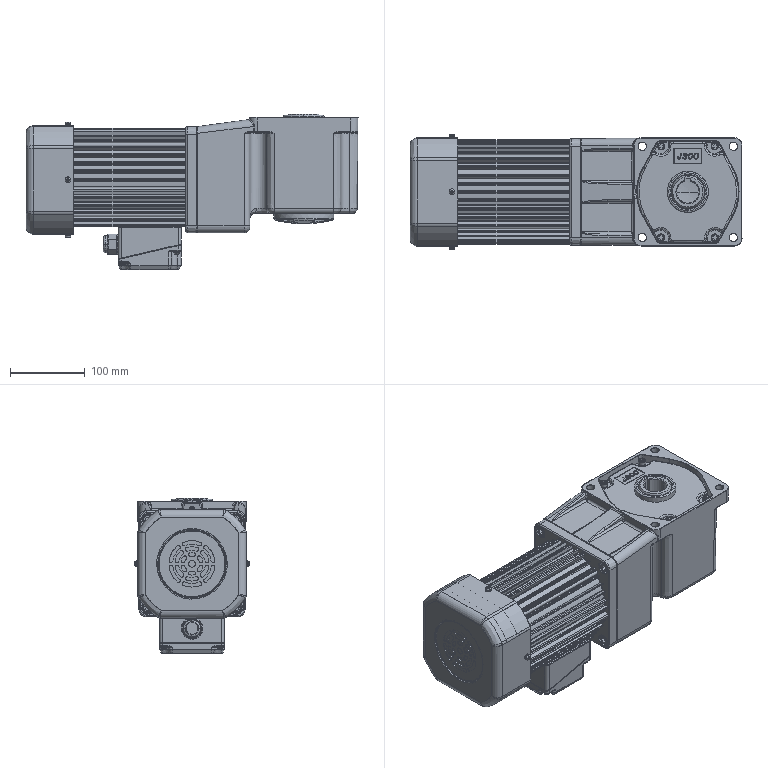Part | STEP file | s750rc-U | 4 solids | 3526 faces | volume 5609613 mm3 | spline 1255 | cylinder 1248 | plane 933 | cone 73 | torus 17 | commonest cylinder face diameters 2 x200 0.4 x158 4 x141 1 x130 8 x48 3 x45